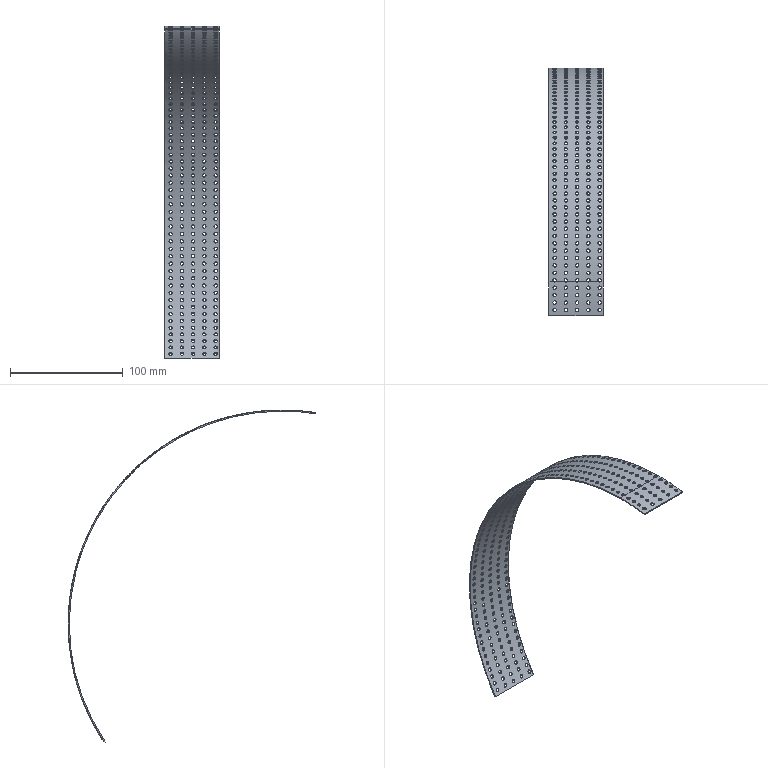Part | STEP file | 09-15 Track inner side plate | 1 solid | 668 faces | box 48 x 220 x 295 mm | volume 18723 mm3 | cylinder 664 | plane 4 | commonest cylinder face diameters 3 x660 378 x2 380 x2